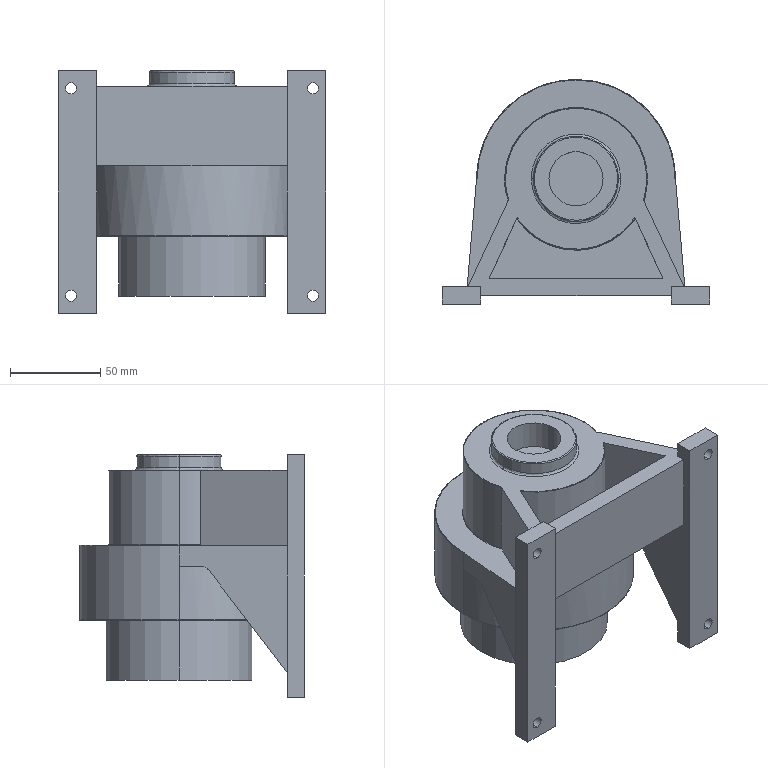Part | STEP file | XWE main body_BWED3922.step | 1 solid | 73 faces | box 148.8 x 124.8 x 134.4 mm | volume 938232 mm3 | plane 36 | cylinder 22 | spline 15 | commonest cylinder face diameters 6.24 x8 78.857 x4 9.6 x2 30 x2 47.314 x2 81.6 x2